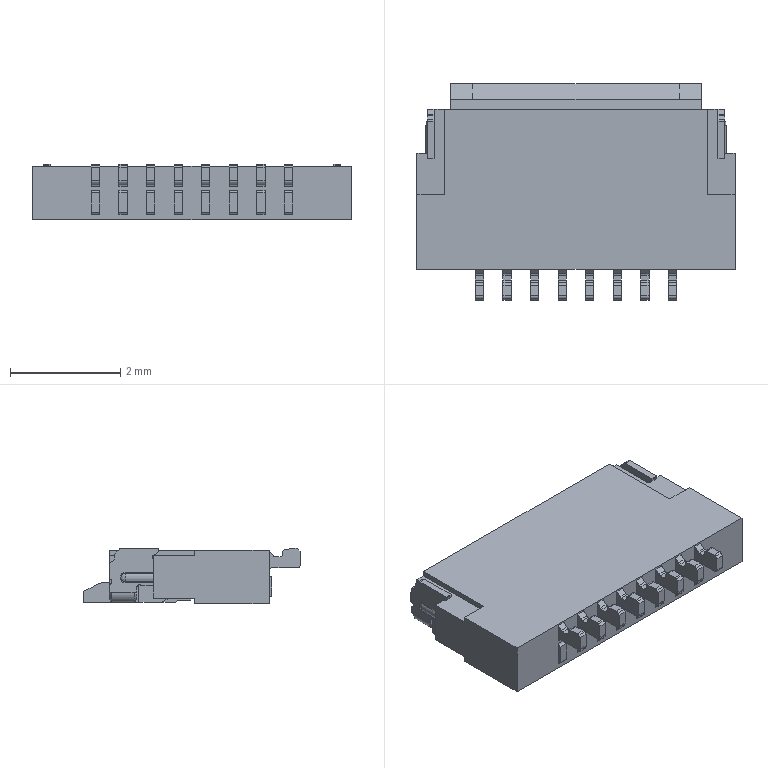Part | Creo | 1 solid | 463 faces | box 5.77 x 3.923 x 1 mm | volume 12.056 mm3 | plane 315 | cylinder 136 | sphere 4 | cone 4 | spline 2 | torus 2 | commonest cylinder face diameters 0.1 x100 0.2 x20 0.04 x4 0.28 x4 0.02 x2 0.125 x2